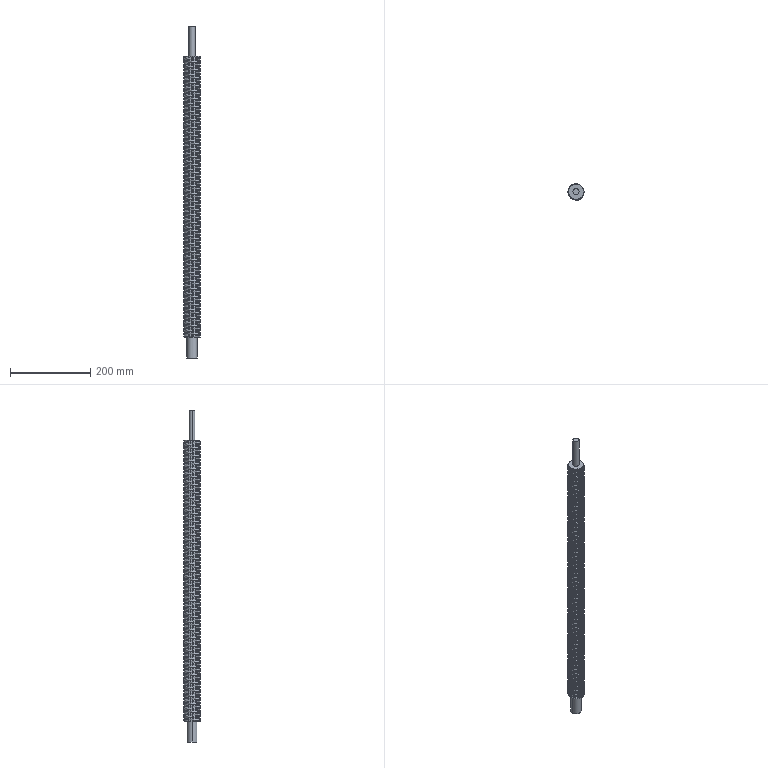Part | SolidWorks | features BaseBody 1 | 1 solid | 371 faces | box 40 x 40 x 825 mm | volume 850730 mm3 | cylinder 355 | spline 12 | plane 4 | commonest cylinder face diameters 40 x351 15 x2 25 x2